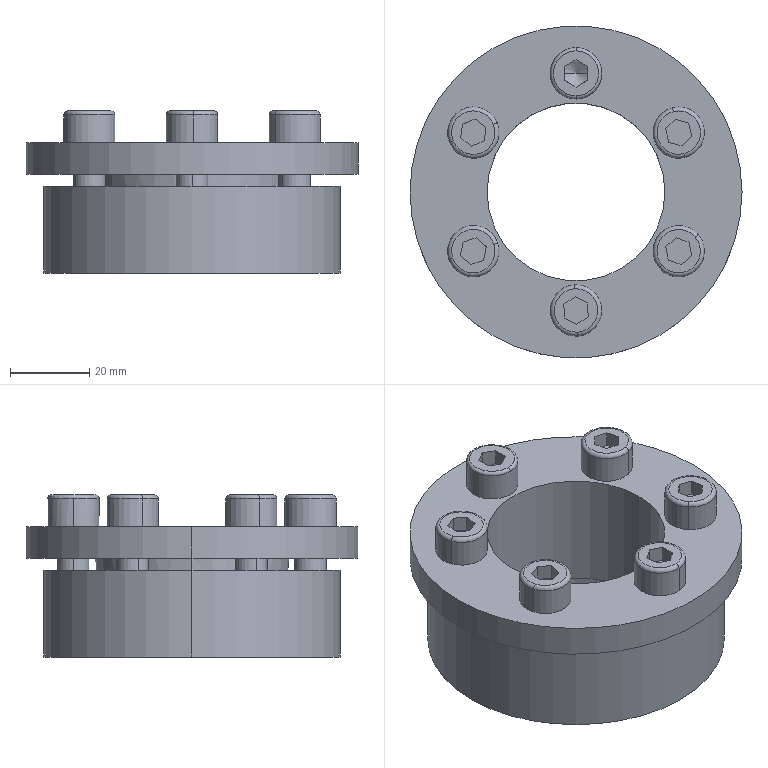Part | SolidWorks | features BaseBody 8 | 8 solids | 160 faces | box 84 x 84 x 41 mm | volume 97003 mm3 | plane 64 | cylinder 54 | torus 24 | cone 18 | commonest cylinder face diameters 6.647 x22 8 x12 13 x12 9 x2 45 x2 75 x2